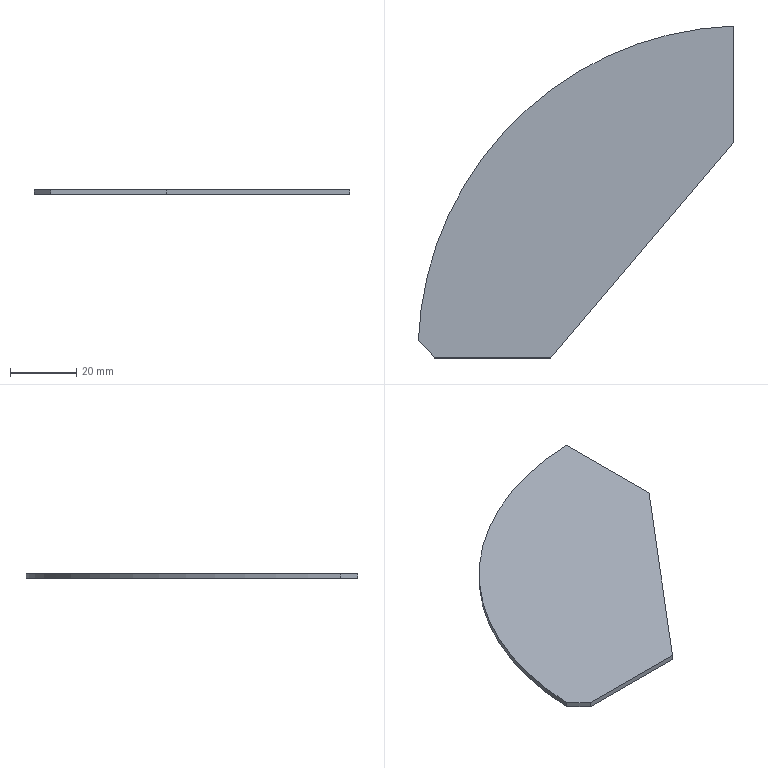Part | STEP file | Box reinforcing rib plate 2001 | 1 solid | 7 faces | box 94.931 x 99.938 x 1.5 mm | volume 8426 mm3 | plane 6 | cylinder 1 | commonest cylinder face diameters 197 x1
STEP:
#1=CARTESIAN_POINT('',(0.,0.,0.));
#2=DIRECTION('',(0.,0.,1.));
#3=DIRECTION('',(1.,0.,0.));
#4=AXIS2_PLACEMENT_3D('',#1,#2,#3);
#5=CARTESIAN_POINT('',(-47.431,-44.813,0.75));
#6=VERTEX_POINT('',#5);
#7=CARTESIAN_POINT('',(47.5,49.938,0.75));
#8=VERTEX_POINT('',#7);
#9=CARTESIAN_POINT('',(51.,-48.5,0.75));
#10=DIRECTION('',(0.,0.,-1.));
#11=DIRECTION('',(-1.,0.,0.));
#12=AXIS2_PLACEMENT_3D('',#9,#10,#11);
#13=CIRCLE('',#12,98.5);
#14=CARTESIAN_POINT('',(0.,0.,0.75));
#15=DIRECTION('',(0.,0.,-1.));
#16=DIRECTION('',(-1.,0.,0.));
#17=AXIS2_PLACEMENT_3D('',#14,#15,#16);
#18=PLANE('',#17);
#19=CARTESIAN_POINT('',(-51.,-48.5));
#20=DIRECTION('',(1.,0.));
#21=AXIS2_PLACEMENT_2D('',#19,#20);
#22=CIRCLE('',#21,98.5);
#23=(GEOMETRIC_REPRESENTATION_CONTEXT(2)PARAMETRIC_REPRESENTATION_CONTEXT()REPRESENTATION_CONTEXT('',''));
#24=DEFINITIONAL_REPRESENTATION('',(#22),#23);
#25=PCURVE('',#18,#24);
#26=CARTESIAN_POINT('',(51.,-48.5,-9.25));
#27=DIRECTION('',(0.,0.,1.));
#28=DIRECTION('',(1.,0.,0.));
#29=AXIS2_PLACEMENT_3D('',#26,#27,#28);
#30=CYLINDRICAL_SURFACE('',#29,98.5);
#31=CARTESIAN_POINT('',(3.142,10.));
#32=DIRECTION('',(-1.,0.));
#33=VECTOR('',#32,1.);
#34=LINE('',#31,#33);
#35=(GEOMETRIC_REPRESENTATION_CONTEXT(2)PARAMETRIC_REPRESENTATION_CONTEXT()REPRESENTATION_CONTEXT('',''));
#36=DEFINITIONAL_REPRESENTATION('',(#34),#35);
#37=PCURVE('',#30,#36);
#38=SURFACE_CURVE('',#13,(#25,#37),.PCURVE_S1.);
#39=EDGE_CURVE('',#6,#8,#38,.T.);
#40=ORIENTED_EDGE('',*,*,#39,.F.);
#41=CARTESIAN_POINT('',(-42.434,-50.,0.75));
#42=VERTEX_POINT('',#41);
#43=CARTESIAN_POINT('',(-42.434,-50.,0.75));
#44=DIRECTION('',(0.6937,-0.7202,0.));
#45=VECTOR('',#44,1.);
#46=LINE('',#43,#45);
#47=CARTESIAN_POINT('',(42.434,-50.));
#48=DIRECTION('',(-0.6937,-0.7202));
#49=VECTOR('',#48,1.);
#50=LINE('',#47,#49);
#51=(GEOMETRIC_REPRESENTATION_CONTEXT(2)PARAMETRIC_REPRESENTATION_CONTEXT()REPRESENTATION_CONTEXT('',''));
#52=DEFINITIONAL_REPRESENTATION('',(#50),#51);
#53=PCURVE('',#18,#52);
#54=CARTESIAN_POINT('',(-42.434,-50.,-9.25));
#55=DIRECTION('',(-0.7202,-0.6937,0.));
#56=DIRECTION('',(0.,0.,1.));
#57=AXIS2_PLACEMENT_3D('',#54,#55,#56);
#58=PLANE('',#57);
#59=CARTESIAN_POINT('',(10.,0.));
#60=DIRECTION('',(0.,-1.));
#61=VECTOR('',#60,1.);
#62=LINE('',#59,#61);
#63=(GEOMETRIC_REPRESENTATION_CONTEXT(2)PARAMETRIC_REPRESENTATION_CONTEXT()REPRESENTATION_CONTEXT('',''));
#64=DEFINITIONAL_REPRESENTATION('',(#62),#63);
#65=PCURVE('',#58,#64);
#66=SURFACE_CURVE('',#46,(#53,#65),.PCURVE_S1.);
#67=EDGE_CURVE('',#6,#42,#66,.T.);
#68=ORIENTED_EDGE('',*,*,#67,.T.);
#69=CARTESIAN_POINT('',(-7.5,-50.,0.75));
#70=VERTEX_POINT('',#69);
#71=CARTESIAN_POINT('',(-47.5,-50.,0.75));
#72=DIRECTION('',(1.,0.,0.));
#73=VECTOR('',#72,1.);
#74=LINE('',#71,#73);
#75=CARTESIAN_POINT('',(47.5,-50.));
#76=DIRECTION('',(-1.,0.));
#77=VECTOR('',#76,1.);
#78=LINE('',#75,#77);
#79=(GEOMETRIC_REPRESENTATION_CONTEXT(2)PARAMETRIC_REPRESENTATION_CONTEXT()REPRESENTATION_CONTEXT('',''));
#80=DEFINITIONAL_REPRESENTATION('',(#78),#79);
#81=PCURVE('',#18,#80);
#82=CARTESIAN_POINT('',(-47.5,-50.,0.75));
#83=DIRECTION('',(0.,1.,0.));
#84=DIRECTION('',(0.,0.,1.));
#85=AXIS2_PLACEMENT_3D('',#82,#83,#84);
#86=PLANE('',#85);
#87=CARTESIAN_POINT('',(0.,0.));
#88=DIRECTION('',(0.,1.));
#89=VECTOR('',#88,1.);
#90=LINE('',#87,#89);
#91=(GEOMETRIC_REPRESENTATION_CONTEXT(2)PARAMETRIC_REPRESENTATION_CONTEXT()REPRESENTATION_CONTEXT('',''));
#92=DEFINITIONAL_REPRESENTATION('',(#90),#91);
#93=PCURVE('',#86,#92);
#94=SURFACE_CURVE('',#74,(#81,#93),.PCURVE_S1.);
#95=EDGE_CURVE('',#42,#70,#94,.T.);
#96=ORIENTED_EDGE('',*,*,#95,.T.);
#97=CARTESIAN_POINT('',(47.5,15.,0.75));
#98=VERTEX_POINT('',#97);
#99=CARTESIAN_POINT('',(-7.5,-50.,0.75));
#100=DIRECTION('',(-0.6459,-0.7634,0.));
#101=VECTOR('',#100,1.);
#102=LINE('',#99,#101);
#103=CARTESIAN_POINT('',(7.5,-50.));
#104=DIRECTION('',(0.6459,-0.7634));
#105=VECTOR('',#104,1.);
#106=LINE('',#103,#105);
#107=(GEOMETRIC_REPRESENTATION_CONTEXT(2)PARAMETRIC_REPRESENTATION_CONTEXT()REPRESENTATION_CONTEXT('',''));
#108=DEFINITIONAL_REPRESENTATION('',(#106),#107);
#109=PCURVE('',#18,#108);
#110=CARTESIAN_POINT('',(-7.5,-50.,-9.25));
#111=DIRECTION('',(-0.7634,0.6459,0.));
#112=DIRECTION('',(-0.6459,-0.7634,0.));
#113=AXIS2_PLACEMENT_3D('',#110,#111,#112);
#114=PLANE('',#113);
#115=CARTESIAN_POINT('',(0.,10.));
#116=DIRECTION('',(1.,0.));
#117=VECTOR('',#116,1.);
#118=LINE('',#115,#117);
#119=(GEOMETRIC_REPRESENTATION_CONTEXT(2)PARAMETRIC_REPRESENTATION_CONTEXT()REPRESENTATION_CONTEXT('',''));
#120=DEFINITIONAL_REPRESENTATION('',(#118),#119);
#121=PCURVE('',#114,#120);
#122=SURFACE_CURVE('',#102,(#109,#121),.PCURVE_S1.);
#123=EDGE_CURVE('',#98,#70,#122,.T.);
#124=ORIENTED_EDGE('',*,*,#123,.F.);
#125=CARTESIAN_POINT('',(47.5,-50.,0.75));
#126=DIRECTION('',(0.,1.,0.));
#127=VECTOR('',#126,1.);
#128=LINE('',#125,#127);
#129=CARTESIAN_POINT('',(-47.5,-50.));
#130=DIRECTION('',(0.,1.));
#131=VECTOR('',#130,1.);
#132=LINE('',#129,#131);
#133=(GEOMETRIC_REPRESENTATION_CONTEXT(2)PARAMETRIC_REPRESENTATION_CONTEXT()REPRESENTATION_CONTEXT('',''));
#134=DEFINITIONAL_REPRESENTATION('',(#132),#133);
#135=PCURVE('',#18,#134);
#136=CARTESIAN_POINT('',(47.5,-50.,0.75));
#137=DIRECTION('',(-1.,0.,0.));
#138=DIRECTION('',(0.,0.,1.));
#139=AXIS2_PLACEMENT_3D('',#136,#137,#138);
#140=PLANE('',#139);
#141=CARTESIAN_POINT('',(0.,0.));
#142=DIRECTION('',(0.,1.));
#143=VECTOR('',#142,1.);
#144=LINE('',#141,#143);
#145=(GEOMETRIC_REPRESENTATION_CONTEXT(2)PARAMETRIC_REPRESENTATION_CONTEXT()REPRESENTATION_CONTEXT('',''));
#146=DEFINITIONAL_REPRESENTATION('',(#144),#145);
#147=PCURVE('',#140,#146);
#148=SURFACE_CURVE('',#128,(#135,#147),.PCURVE_S1.);
#149=EDGE_CURVE('',#98,#8,#148,.T.);
#150=ORIENTED_EDGE('',*,*,#149,.T.);
#151=EDGE_LOOP('',(#40,#68,#96,#124,#150));
#152=FACE_BOUND('',#151,.T.);
#153=ADVANCED_FACE('',(#152),#18,.F.);
#154=CARTESIAN_POINT('',(-42.434,-50.,-0.75));
#155=VERTEX_POINT('',#154);
#156=CARTESIAN_POINT('',(-7.5,-50.,-0.75));
#157=VERTEX_POINT('',#156);
#158=CARTESIAN_POINT('',(-47.5,-50.,-0.75));
#159=DIRECTION('',(1.,0.,0.));
#160=VECTOR('',#159,1.);
#161=LINE('',#158,#160);
#162=CARTESIAN_POINT('',(0.,0.,-0.75));
#163=DIRECTION('',(0.,0.,-1.));
#164=DIRECTION('',(-1.,0.,0.));
#165=AXIS2_PLACEMENT_3D('',#162,#163,#164);
#166=PLANE('',#165);
#167=CARTESIAN_POINT('',(47.5,-50.));
#168=DIRECTION('',(-1.,0.));
#169=VECTOR('',#168,1.);
#170=LINE('',#167,#169);
#171=(GEOMETRIC_REPRESENTATION_CONTEXT(2)PARAMETRIC_REPRESENTATION_CONTEXT()REPRESENTATION_CONTEXT('',''));
#172=DEFINITIONAL_REPRESENTATION('',(#170),#171);
#173=PCURVE('',#166,#172);
#174=CARTESIAN_POINT('',(-1.5,0.));
#175=DIRECTION('',(0.,1.));
#176=VECTOR('',#175,1.);
#177=LINE('',#174,#176);
#178=(GEOMETRIC_REPRESENTATION_CONTEXT(2)PARAMETRIC_REPRESENTATION_CONTEXT()REPRESENTATION_CONTEXT('',''));
#179=DEFINITIONAL_REPRESENTATION('',(#177),#178);
#180=PCURVE('',#86,#179);
#181=SURFACE_CURVE('',#161,(#173,#180),.PCURVE_S1.);
#182=EDGE_CURVE('',#155,#157,#181,.T.);
#183=ORIENTED_EDGE('',*,*,#182,.F.);
#184=CARTESIAN_POINT('',(-47.431,-44.813,-0.75));
#185=VERTEX_POINT('',#184);
#186=CARTESIAN_POINT('',(-46.994,-45.267,-0.75));
#187=DIRECTION('',(-0.6937,0.7202,0.));
#188=VECTOR('',#187,1.);
#189=LINE('',#186,#188);
#190=CARTESIAN_POINT('',(46.994,-45.267));
#191=DIRECTION('',(0.6937,0.7202));
#192=VECTOR('',#191,1.);
#193=LINE('',#190,#192);
#194=(GEOMETRIC_REPRESENTATION_CONTEXT(2)PARAMETRIC_REPRESENTATION_CONTEXT()REPRESENTATION_CONTEXT('',''));
#195=DEFINITIONAL_REPRESENTATION('',(#193),#194);
#196=PCURVE('',#166,#195);
#197=CARTESIAN_POINT('',(8.5,6.572));
#198=DIRECTION('',(0.,1.));
#199=VECTOR('',#198,1.);
#200=LINE('',#197,#199);
#201=(GEOMETRIC_REPRESENTATION_CONTEXT(2)PARAMETRIC_REPRESENTATION_CONTEXT()REPRESENTATION_CONTEXT('',''));
#202=DEFINITIONAL_REPRESENTATION('',(#200),#201);
#203=PCURVE('',#58,#202);
#204=SURFACE_CURVE('',#189,(#196,#203),.PCURVE_S1.);
#205=EDGE_CURVE('',#155,#185,#204,.T.);
#206=ORIENTED_EDGE('',*,*,#205,.T.);
#207=CARTESIAN_POINT('',(47.5,49.938,-0.75));
#208=VERTEX_POINT('',#207);
#209=CARTESIAN_POINT('',(51.,-48.5,-0.75));
#210=DIRECTION('',(0.,0.,1.));
#211=DIRECTION('',(-1.,0.,0.));
#212=AXIS2_PLACEMENT_3D('',#209,#210,#211);
#213=CIRCLE('',#212,98.5);
#214=CARTESIAN_POINT('',(47.5,-48.5));
#215=CARTESIAN_POINT('',(47.5,-219.107));
#216=CARTESIAN_POINT('',(-100.25,-133.804));
#217=CARTESIAN_POINT('',(-248.,-48.5));
#218=CARTESIAN_POINT('',(-100.25,36.804));
#219=CARTESIAN_POINT('',(47.5,122.107));
#220=CARTESIAN_POINT('',(47.5,-48.5));
#221=(BOUNDED_CURVE()B_SPLINE_CURVE(2,(#214,#215,#216,#217,#218,#219,#220),.UNSPECIFIED.,.T.,.F.)B_SPLINE_CURVE_WITH_KNOTS((1,2,2,2,2,1),(-2.094,0.,2.094,4.189,6.283,8.378),.UNSPECIFIED.)CURVE()GEOMETRIC_REPRESENTATION_ITEM()RATIONAL_B_SPLINE_CURVE((1.,0.5,1.,0.5,1.,0.5,1.))REPRESENTATION_ITEM(''));
#222=(GEOMETRIC_REPRESENTATION_CONTEXT(2)PARAMETRIC_REPRESENTATION_CONTEXT()REPRESENTATION_CONTEXT('',''));
#223=DEFINITIONAL_REPRESENTATION('',(#221),#222);
#224=PCURVE('',#166,#223);
#225=CARTESIAN_POINT('',(-3.142,8.5));
#226=DIRECTION('',(1.,0.));
#227=VECTOR('',#226,1.);
#228=LINE('',#225,#227);
#229=(GEOMETRIC_REPRESENTATION_CONTEXT(2)PARAMETRIC_REPRESENTATION_CONTEXT()REPRESENTATION_CONTEXT('',''));
#230=DEFINITIONAL_REPRESENTATION('',(#228),#229);
#231=PCURVE('',#30,#230);
#232=SURFACE_CURVE('',#213,(#224,#231),.PCURVE_S1.);
#233=EDGE_CURVE('',#208,#185,#232,.T.);
#234=ORIENTED_EDGE('',*,*,#233,.F.);
#235=CARTESIAN_POINT('',(47.5,15.,-0.75));
#236=VERTEX_POINT('',#235);
#237=CARTESIAN_POINT('',(47.5,-50.,-0.75));
#238=DIRECTION('',(0.,1.,0.));
#239=VECTOR('',#238,1.);
#240=LINE('',#237,#239);
#241=CARTESIAN_POINT('',(-47.5,-50.));
#242=DIRECTION('',(0.,1.));
#243=VECTOR('',#242,1.);
#244=LINE('',#241,#243);
#245=(GEOMETRIC_REPRESENTATION_CONTEXT(2)PARAMETRIC_REPRESENTATION_CONTEXT()REPRESENTATION_CONTEXT('',''));
#246=DEFINITIONAL_REPRESENTATION('',(#244),#245);
#247=PCURVE('',#166,#246);
#248=CARTESIAN_POINT('',(-1.5,0.));
#249=DIRECTION('',(0.,1.));
#250=VECTOR('',#249,1.);
#251=LINE('',#248,#250);
#252=(GEOMETRIC_REPRESENTATION_CONTEXT(2)PARAMETRIC_REPRESENTATION_CONTEXT()REPRESENTATION_CONTEXT('',''));
#253=DEFINITIONAL_REPRESENTATION('',(#251),#252);
#254=PCURVE('',#140,#253);
#255=SURFACE_CURVE('',#240,(#247,#254),.PCURVE_S1.);
#256=EDGE_CURVE('',#236,#208,#255,.T.);
#257=ORIENTED_EDGE('',*,*,#256,.F.);
#258=CARTESIAN_POINT('',(20.284,-17.164,-0.75));
#259=DIRECTION('',(0.6459,0.7634,0.));
#260=VECTOR('',#259,1.);
#261=LINE('',#258,#260);
#262=CARTESIAN_POINT('',(-20.284,-17.164));
#263=DIRECTION('',(-0.6459,0.7634));
#264=VECTOR('',#263,1.);
#265=LINE('',#262,#264);
#266=(GEOMETRIC_REPRESENTATION_CONTEXT(2)PARAMETRIC_REPRESENTATION_CONTEXT()REPRESENTATION_CONTEXT('',''));
#267=DEFINITIONAL_REPRESENTATION('',(#265),#266);
#268=PCURVE('',#166,#267);
#269=CARTESIAN_POINT('',(-43.014,8.5));
#270=DIRECTION('',(-1.,0.));
#271=VECTOR('',#270,1.);
#272=LINE('',#269,#271);
#273=(GEOMETRIC_REPRESENTATION_CONTEXT(2)PARAMETRIC_REPRESENTATION_CONTEXT()REPRESENTATION_CONTEXT('',''));
#274=DEFINITIONAL_REPRESENTATION('',(#272),#273);
#275=PCURVE('',#114,#274);
#276=SURFACE_CURVE('',#261,(#268,#275),.PCURVE_S1.);
#277=EDGE_CURVE('',#157,#236,#276,.T.);
#278=ORIENTED_EDGE('',*,*,#277,.F.);
#279=EDGE_LOOP('',(#183,#206,#234,#257,#278));
#280=FACE_BOUND('',#279,.T.);
#281=ADVANCED_FACE('',(#280),#166,.T.);
#282=ORIENTED_EDGE('',*,*,#149,.F.);
#283=CARTESIAN_POINT('',(47.5,15.,-9.25));
#284=DIRECTION('',(0.,0.,1.));
#285=VECTOR('',#284,1.);
#286=LINE('',#283,#285);
#287=CARTESIAN_POINT('',(-10.,65.));
#288=DIRECTION('',(1.,0.));
#289=VECTOR('',#288,1.);
#290=LINE('',#287,#289);
#291=(GEOMETRIC_REPRESENTATION_CONTEXT(2)PARAMETRIC_REPRESENTATION_CONTEXT()REPRESENTATION_CONTEXT('',''));
#292=DEFINITIONAL_REPRESENTATION('',(#290),#291);
#293=PCURVE('',#140,#292);
#294=CARTESIAN_POINT('',(-85.147,0.));
#295=DIRECTION('',(0.,1.));
#296=VECTOR('',#295,1.);
#297=LINE('',#294,#296);
#298=(GEOMETRIC_REPRESENTATION_CONTEXT(2)PARAMETRIC_REPRESENTATION_CONTEXT()REPRESENTATION_CONTEXT('',''));
#299=DEFINITIONAL_REPRESENTATION('',(#297),#298);
#300=PCURVE('',#114,#299);
#301=SURFACE_CURVE('',#286,(#293,#300),.PCURVE_S1.);
#302=EDGE_CURVE('',#236,#98,#301,.T.);
#303=ORIENTED_EDGE('',*,*,#302,.F.);
#304=ORIENTED_EDGE('',*,*,#256,.T.);
#305=CARTESIAN_POINT('',(47.5,49.938,-9.25));
#306=DIRECTION('',(0.,0.,1.));
#307=VECTOR('',#306,1.);
#308=LINE('',#305,#307);
#309=CARTESIAN_POINT('',(-10.,99.938));
#310=DIRECTION('',(1.,0.));
#311=VECTOR('',#310,1.);
#312=LINE('',#309,#311);
#313=(GEOMETRIC_REPRESENTATION_CONTEXT(2)PARAMETRIC_REPRESENTATION_CONTEXT()REPRESENTATION_CONTEXT('',''));
#314=DEFINITIONAL_REPRESENTATION('',(#312),#313);
#315=PCURVE('',#140,#314);
#316=CARTESIAN_POINT('',(1.606,0.));
#317=DIRECTION('',(0.,1.));
#318=VECTOR('',#317,1.);
#319=LINE('',#316,#318);
#320=(GEOMETRIC_REPRESENTATION_CONTEXT(2)PARAMETRIC_REPRESENTATION_CONTEXT()REPRESENTATION_CONTEXT('',''));
#321=DEFINITIONAL_REPRESENTATION('',(#319),#320);
#322=PCURVE('',#30,#321);
#323=SURFACE_CURVE('',#308,(#315,#322),.PCURVE_S1.);
#324=EDGE_CURVE('',#208,#8,#323,.T.);
#325=ORIENTED_EDGE('',*,*,#324,.T.);
#326=EDGE_LOOP('',(#282,#303,#304,#325));
#327=FACE_BOUND('',#326,.T.);
#328=ADVANCED_FACE('',(#327),#140,.F.);
#329=ORIENTED_EDGE('',*,*,#95,.F.);
#330=CARTESIAN_POINT('',(-42.434,-50.,0.75));
#331=DIRECTION('',(0.,0.,-1.));
#332=VECTOR('',#331,1.);
#333=LINE('',#330,#332);
#334=CARTESIAN_POINT('',(0.,5.066));
#335=DIRECTION('',(-1.,0.));
#336=VECTOR('',#335,1.);
#337=LINE('',#334,#336);
#338=(GEOMETRIC_REPRESENTATION_CONTEXT(2)PARAMETRIC_REPRESENTATION_CONTEXT()REPRESENTATION_CONTEXT('',''));
#339=DEFINITIONAL_REPRESENTATION('',(#337),#338);
#340=PCURVE('',#86,#339);
#341=CARTESIAN_POINT('',(10.,0.));
#342=DIRECTION('',(-1.,0.));
#343=VECTOR('',#342,1.);
#344=LINE('',#341,#343);
#345=(GEOMETRIC_REPRESENTATION_CONTEXT(2)PARAMETRIC_REPRESENTATION_CONTEXT()REPRESENTATION_CONTEXT('',''));
#346=DEFINITIONAL_REPRESENTATION('',(#344),#345);
#347=PCURVE('',#58,#346);
#348=SURFACE_CURVE('',#333,(#340,#347),.PCURVE_S1.);
#349=EDGE_CURVE('',#42,#155,#348,.T.);
#350=ORIENTED_EDGE('',*,*,#349,.T.);
#351=ORIENTED_EDGE('',*,*,#182,.T.);
#352=CARTESIAN_POINT('',(-7.5,-50.,-9.25));
#353=DIRECTION('',(0.,0.,1.));
#354=VECTOR('',#353,1.);
#355=LINE('',#352,#354);
#356=CARTESIAN_POINT('',(-10.,40.));
#357=DIRECTION('',(1.,0.));
#358=VECTOR('',#357,1.);
#359=LINE('',#356,#358);
#360=(GEOMETRIC_REPRESENTATION_CONTEXT(2)PARAMETRIC_REPRESENTATION_CONTEXT()REPRESENTATION_CONTEXT('',''));
#361=DEFINITIONAL_REPRESENTATION('',(#359),#360);
#362=PCURVE('',#86,#361);
#363=CARTESIAN_POINT('',(0.,0.));
#364=DIRECTION('',(0.,1.));
#365=VECTOR('',#364,1.);
#366=LINE('',#363,#365);
#367=(GEOMETRIC_REPRESENTATION_CONTEXT(2)PARAMETRIC_REPRESENTATION_CONTEXT()REPRESENTATION_CONTEXT('',''));
#368=DEFINITIONAL_REPRESENTATION('',(#366),#367);
#369=PCURVE('',#114,#368);
#370=SURFACE_CURVE('',#355,(#362,#369),.PCURVE_S1.);
#371=EDGE_CURVE('',#157,#70,#370,.T.);
#372=ORIENTED_EDGE('',*,*,#371,.T.);
#373=EDGE_LOOP('',(#329,#350,#351,#372));
#374=FACE_BOUND('',#373,.T.);
#375=ADVANCED_FACE('',(#374),#86,.F.);
#376=ORIENTED_EDGE('',*,*,#233,.T.);
#377=CARTESIAN_POINT('',(-47.431,-44.813,-9.25));
#378=DIRECTION('',(0.,0.,1.));
#379=VECTOR('',#378,1.);
#380=LINE('',#377,#379);
#381=CARTESIAN_POINT('',(3.104,0.));
#382=DIRECTION('',(0.,1.));
#383=VECTOR('',#382,1.);
#384=LINE('',#381,#383);
#385=(GEOMETRIC_REPRESENTATION_CONTEXT(2)PARAMETRIC_REPRESENTATION_CONTEXT()REPRESENTATION_CONTEXT('',''));
#386=DEFINITIONAL_REPRESENTATION('',(#384),#385);
#387=PCURVE('',#30,#386);
#388=CARTESIAN_POINT('',(0.,7.202));
#389=DIRECTION('',(1.,0.));
#390=VECTOR('',#389,1.);
#391=LINE('',#388,#390);
#392=(GEOMETRIC_REPRESENTATION_CONTEXT(2)PARAMETRIC_REPRESENTATION_CONTEXT()REPRESENTATION_CONTEXT('',''));
#393=DEFINITIONAL_REPRESENTATION('',(#391),#392);
#394=PCURVE('',#58,#393);
#395=SURFACE_CURVE('',#380,(#387,#394),.PCURVE_S1.);
#396=EDGE_CURVE('',#185,#6,#395,.T.);
#397=ORIENTED_EDGE('',*,*,#396,.T.);
#398=ORIENTED_EDGE('',*,*,#39,.T.);
#399=ORIENTED_EDGE('',*,*,#324,.F.);
#400=EDGE_LOOP('',(#376,#397,#398,#399));
#401=FACE_BOUND('',#400,.T.);
#402=ADVANCED_FACE('',(#401),#30,.T.);
#403=ORIENTED_EDGE('',*,*,#277,.T.);
#404=ORIENTED_EDGE('',*,*,#302,.T.);
#405=ORIENTED_EDGE('',*,*,#123,.T.);
#406=ORIENTED_EDGE('',*,*,#371,.F.);
#407=EDGE_LOOP('',(#403,#404,#405,#406));
#408=FACE_BOUND('',#407,.T.);
#409=ADVANCED_FACE('',(#408),#114,.F.);
#410=ORIENTED_EDGE('',*,*,#67,.F.);
#411=ORIENTED_EDGE('',*,*,#396,.F.);
#412=ORIENTED_EDGE('',*,*,#205,.F.);
#413=ORIENTED_EDGE('',*,*,#349,.F.);
#414=EDGE_LOOP('',(#410,#411,#412,#413));
#415=FACE_BOUND('',#414,.T.);
#416=ADVANCED_FACE('',(#415),#58,.T.);
#417=CLOSED_SHELL('',(#153,#281,#328,#375,#402,#409,#416));
#418=MANIFOLD_SOLID_BREP('',#417);
#419=(LENGTH_UNIT()NAMED_UNIT(*)SI_UNIT(.MILLI.,.METRE.));
#420=UNCERTAINTY_MEASURE_WITH_UNIT(LENGTH_MEASURE(0.0000001),#419,'','');
#421=(NAMED_UNIT(*)PLANE_ANGLE_UNIT()SI_UNIT($,.RADIAN.));
#422=(NAMED_UNIT(*)SI_UNIT($,.STERADIAN.)SOLID_ANGLE_UNIT());
#423=(GEOMETRIC_REPRESENTATION_CONTEXT(3)GLOBAL_UNCERTAINTY_ASSIGNED_CONTEXT((#420))GLOBAL_UNIT_ASSIGNED_CONTEXT((#419,#421,#422))REPRESENTATION_CONTEXT('',''));
#424=ADVANCED_BREP_SHAPE_REPRESENTATION('',(#4,#418),#423);